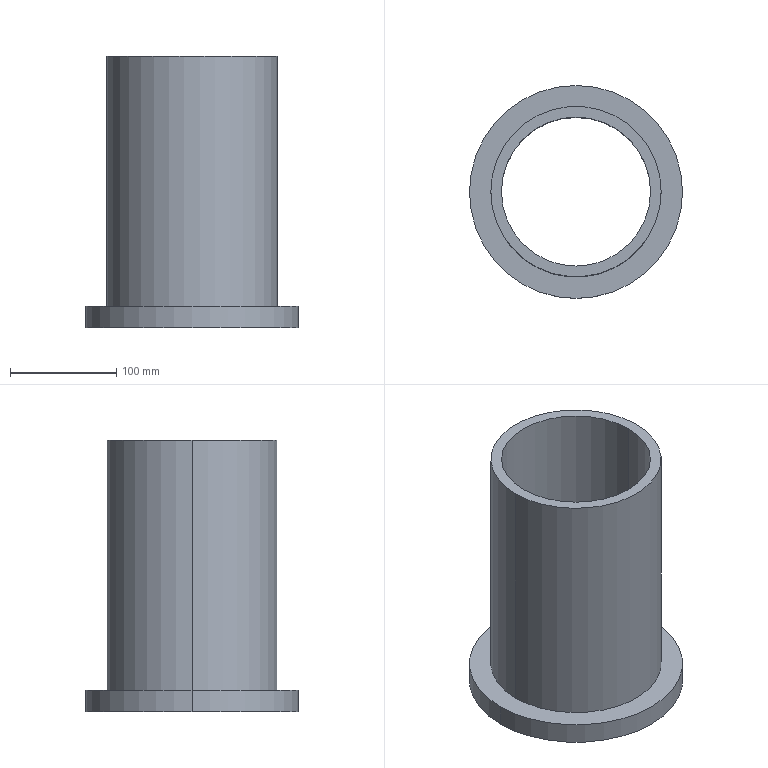Part | SolidWorks | features BaseBody 1 | 1 solid | 9 faces | box 200 x 200 x 255 mm | volume 1427854 mm3 | cylinder 6 | plane 3 | commonest cylinder face diameters 140 x2 160 x2 200 x2
STEP:
#1=CARTESIAN_POINT('',(335.077,953.249,-384.893));
#2=VERTEX_POINT('',#1);
#3=CARTESIAN_POINT('',(335.077,953.249,-639.893));
#4=VERTEX_POINT('',#3);
#5=CARTESIAN_POINT('',(335.077,953.249,-384.893));
#6=DIRECTION('',(0.,0.,-1.));
#7=VECTOR('',#6,1000.);
#8=LINE('',#5,#7);
#9=EDGE_CURVE('',#2,#4,#8,.T.);
#10=ORIENTED_EDGE('',*,*,#9,.F.);
#11=CARTESIAN_POINT('',(195.077,953.249,-384.893));
#12=VERTEX_POINT('',#11);
#13=CARTESIAN_POINT('',(265.077,953.249,-384.893));
#14=DIRECTION('',(0.,0.,1.));
#15=DIRECTION('',(1.,0.,0.));
#16=AXIS2_PLACEMENT_3D('',#13,#14,#15);
#17=CIRCLE('',#16,70.);
#18=EDGE_CURVE('',#2,#12,#17,.T.);
#19=ORIENTED_EDGE('',*,*,#18,.T.);
#20=CARTESIAN_POINT('',(195.077,953.249,-639.893));
#21=VERTEX_POINT('',#20);
#22=CARTESIAN_POINT('',(195.077,953.249,-384.893));
#23=DIRECTION('',(0.,0.,-1.));
#24=VECTOR('',#23,1000.);
#25=LINE('',#22,#24);
#26=EDGE_CURVE('',#12,#21,#25,.T.);
#27=ORIENTED_EDGE('',*,*,#26,.T.);
#28=CARTESIAN_POINT('',(265.077,953.249,-639.893));
#29=DIRECTION('',(0.,0.,1.));
#30=DIRECTION('',(1.,0.,0.));
#31=AXIS2_PLACEMENT_3D('',#28,#29,#30);
#32=CIRCLE('',#31,70.);
#33=EDGE_CURVE('',#4,#21,#32,.T.);
#34=ORIENTED_EDGE('',*,*,#33,.F.);
#35=EDGE_LOOP('',(#10,#19,#27,#34));
#36=FACE_OUTER_BOUND('',#35,.T.);
#37=CARTESIAN_POINT('',(265.077,953.249,-384.893));
#38=DIRECTION('',(0.,0.,-1.));
#39=DIRECTION('',(1.,0.,0.));
#40=AXIS2_PLACEMENT_3D('',#37,#38,#39);
#41=CYLINDRICAL_SURFACE('',#40,70.);
#42=ADVANCED_FACE('',(#36),#41,.F.);
#43=CARTESIAN_POINT('',(345.077,953.249,-384.893));
#44=VERTEX_POINT('',#43);
#45=CARTESIAN_POINT('',(345.077,953.249,-619.893));
#46=VERTEX_POINT('',#45);
#47=CARTESIAN_POINT('',(345.077,953.249,-384.893));
#48=DIRECTION('',(0.,0.,-1.));
#49=VECTOR('',#48,1000.);
#50=LINE('',#47,#49);
#51=EDGE_CURVE('',#44,#46,#50,.T.);
#52=ORIENTED_EDGE('',*,*,#51,.F.);
#53=CARTESIAN_POINT('',(185.077,953.249,-384.893));
#54=VERTEX_POINT('',#53);
#55=CARTESIAN_POINT('',(265.077,953.249,-384.893));
#56=DIRECTION('',(0.,0.,1.));
#57=DIRECTION('',(1.,0.,0.));
#58=AXIS2_PLACEMENT_3D('',#55,#56,#57);
#59=CIRCLE('',#58,80.);
#60=EDGE_CURVE('',#54,#44,#59,.T.);
#61=ORIENTED_EDGE('',*,*,#60,.F.);
#62=CARTESIAN_POINT('',(185.077,953.249,-619.893));
#63=VERTEX_POINT('',#62);
#64=CARTESIAN_POINT('',(185.077,953.249,-384.893));
#65=DIRECTION('',(0.,0.,-1.));
#66=VECTOR('',#65,1000.);
#67=LINE('',#64,#66);
#68=EDGE_CURVE('',#54,#63,#67,.T.);
#69=ORIENTED_EDGE('',*,*,#68,.T.);
#70=CARTESIAN_POINT('',(265.077,953.249,-619.893));
#71=DIRECTION('',(0.,0.,-1.));
#72=DIRECTION('',(1.,0.,0.));
#73=AXIS2_PLACEMENT_3D('',#70,#71,#72);
#74=CIRCLE('',#73,80.);
#75=EDGE_CURVE('',#46,#63,#74,.T.);
#76=ORIENTED_EDGE('',*,*,#75,.F.);
#77=EDGE_LOOP('',(#52,#61,#69,#76));
#78=FACE_OUTER_BOUND('',#77,.T.);
#79=CARTESIAN_POINT('',(265.077,953.249,-384.893));
#80=DIRECTION('',(0.,0.,-1.));
#81=DIRECTION('',(1.,0.,0.));
#82=AXIS2_PLACEMENT_3D('',#79,#80,#81);
#83=CYLINDRICAL_SURFACE('',#82,80.);
#84=ADVANCED_FACE('',(#78),#83,.T.);
#85=CARTESIAN_POINT('',(265.077,953.249,-384.893));
#86=DIRECTION('',(0.,0.,1.));
#87=DIRECTION('',(1.,0.,0.));
#88=AXIS2_PLACEMENT_3D('',#85,#86,#87);
#89=CIRCLE('',#88,70.);
#90=EDGE_CURVE('',#12,#2,#89,.T.);
#91=ORIENTED_EDGE('',*,*,#90,.F.);
#92=ORIENTED_EDGE('',*,*,#18,.F.);
#93=EDGE_LOOP('',(#91,#92));
#94=FACE_BOUND('',#93,.T.);
#95=ORIENTED_EDGE('',*,*,#60,.T.);
#96=CARTESIAN_POINT('',(265.077,953.249,-384.893));
#97=DIRECTION('',(0.,0.,1.));
#98=DIRECTION('',(1.,0.,0.));
#99=AXIS2_PLACEMENT_3D('',#96,#97,#98);
#100=CIRCLE('',#99,80.);
#101=EDGE_CURVE('',#44,#54,#100,.T.);
#102=ORIENTED_EDGE('',*,*,#101,.T.);
#103=EDGE_LOOP('',(#95,#102));
#104=FACE_OUTER_BOUND('',#103,.T.);
#105=CARTESIAN_POINT('',(265.077,953.249,-384.893));
#106=DIRECTION('',(0.,0.,1.));
#107=DIRECTION('',(1.,0.,0.));
#108=AXIS2_PLACEMENT_3D('',#105,#106,#107);
#109=PLANE('',#108);
#110=ADVANCED_FACE('',(#94,#104),#109,.T.);
#111=CARTESIAN_POINT('',(365.077,953.249,-619.893));
#112=VERTEX_POINT('',#111);
#113=CARTESIAN_POINT('',(365.077,953.249,-639.893));
#114=VERTEX_POINT('',#113);
#115=CARTESIAN_POINT('',(365.077,953.249,-619.893));
#116=DIRECTION('',(0.,0.,-1.));
#117=VECTOR('',#116,1000.);
#118=LINE('',#115,#117);
#119=EDGE_CURVE('',#112,#114,#118,.T.);
#120=ORIENTED_EDGE('',*,*,#119,.F.);
#121=CARTESIAN_POINT('',(165.077,953.249,-619.893));
#122=VERTEX_POINT('',#121);
#123=CARTESIAN_POINT('',(265.077,953.249,-619.893));
#124=DIRECTION('',(0.,0.,1.));
#125=DIRECTION('',(1.,0.,0.));
#126=AXIS2_PLACEMENT_3D('',#123,#124,#125);
#127=CIRCLE('',#126,100.);
#128=EDGE_CURVE('',#122,#112,#127,.T.);
#129=ORIENTED_EDGE('',*,*,#128,.F.);
#130=CARTESIAN_POINT('',(165.077,953.249,-639.893));
#131=VERTEX_POINT('',#130);
#132=CARTESIAN_POINT('',(165.077,953.249,-619.893));
#133=DIRECTION('',(0.,0.,-1.));
#134=VECTOR('',#133,1000.);
#135=LINE('',#132,#134);
#136=EDGE_CURVE('',#122,#131,#135,.T.);
#137=ORIENTED_EDGE('',*,*,#136,.T.);
#138=CARTESIAN_POINT('',(265.077,953.249,-639.893));
#139=DIRECTION('',(0.,0.,1.));
#140=DIRECTION('',(1.,0.,0.));
#141=AXIS2_PLACEMENT_3D('',#138,#139,#140);
#142=CIRCLE('',#141,100.);
#143=EDGE_CURVE('',#131,#114,#142,.T.);
#144=ORIENTED_EDGE('',*,*,#143,.T.);
#145=EDGE_LOOP('',(#120,#129,#137,#144));
#146=FACE_OUTER_BOUND('',#145,.T.);
#147=CARTESIAN_POINT('',(265.077,953.249,-619.893));
#148=DIRECTION('',(0.,0.,-1.));
#149=DIRECTION('',(1.,0.,0.));
#150=AXIS2_PLACEMENT_3D('',#147,#148,#149);
#151=CYLINDRICAL_SURFACE('',#150,100.);
#152=ADVANCED_FACE('',(#146),#151,.T.);
#153=CARTESIAN_POINT('',(265.077,953.249,-619.893));
#154=DIRECTION('',(0.,0.,-1.));
#155=DIRECTION('',(1.,0.,0.));
#156=AXIS2_PLACEMENT_3D('',#153,#154,#155);
#157=CIRCLE('',#156,80.);
#158=EDGE_CURVE('',#63,#46,#157,.T.);
#159=ORIENTED_EDGE('',*,*,#158,.T.);
#160=ORIENTED_EDGE('',*,*,#75,.T.);
#161=EDGE_LOOP('',(#159,#160));
#162=FACE_BOUND('',#161,.T.);
#163=ORIENTED_EDGE('',*,*,#128,.T.);
#164=CARTESIAN_POINT('',(265.077,953.249,-619.893));
#165=DIRECTION('',(0.,0.,1.));
#166=DIRECTION('',(1.,0.,0.));
#167=AXIS2_PLACEMENT_3D('',#164,#165,#166);
#168=CIRCLE('',#167,100.);
#169=EDGE_CURVE('',#112,#122,#168,.T.);
#170=ORIENTED_EDGE('',*,*,#169,.T.);
#171=EDGE_LOOP('',(#163,#170));
#172=FACE_OUTER_BOUND('',#171,.T.);
#173=CARTESIAN_POINT('',(265.077,953.249,-619.893));
#174=DIRECTION('',(0.,0.,1.));
#175=DIRECTION('',(1.,0.,0.));
#176=AXIS2_PLACEMENT_3D('',#173,#174,#175);
#177=PLANE('',#176);
#178=ADVANCED_FACE('',(#162,#172),#177,.T.);
#179=CARTESIAN_POINT('',(265.077,953.249,-639.893));
#180=DIRECTION('',(0.,0.,1.));
#181=DIRECTION('',(1.,0.,0.));
#182=AXIS2_PLACEMENT_3D('',#179,#180,#181);
#183=CIRCLE('',#182,70.);
#184=EDGE_CURVE('',#21,#4,#183,.T.);
#185=ORIENTED_EDGE('',*,*,#184,.T.);
#186=ORIENTED_EDGE('',*,*,#33,.T.);
#187=EDGE_LOOP('',(#185,#186));
#188=FACE_BOUND('',#187,.T.);
#189=ORIENTED_EDGE('',*,*,#143,.F.);
#190=CARTESIAN_POINT('',(265.077,953.249,-639.893));
#191=DIRECTION('',(0.,0.,1.));
#192=DIRECTION('',(1.,0.,0.));
#193=AXIS2_PLACEMENT_3D('',#190,#191,#192);
#194=CIRCLE('',#193,100.);
#195=EDGE_CURVE('',#114,#131,#194,.T.);
#196=ORIENTED_EDGE('',*,*,#195,.F.);
#197=EDGE_LOOP('',(#189,#196));
#198=FACE_OUTER_BOUND('',#197,.T.);
#199=CARTESIAN_POINT('',(265.077,953.249,-639.893));
#200=DIRECTION('',(0.,0.,1.));
#201=DIRECTION('',(1.,0.,0.));
#202=AXIS2_PLACEMENT_3D('',#199,#200,#201);
#203=PLANE('',#202);
#204=ADVANCED_FACE('',(#188,#198),#203,.F.);
#205=ORIENTED_EDGE('',*,*,#169,.F.);
#206=ORIENTED_EDGE('',*,*,#119,.T.);
#207=ORIENTED_EDGE('',*,*,#195,.T.);
#208=ORIENTED_EDGE('',*,*,#136,.F.);
#209=EDGE_LOOP('',(#205,#206,#207,#208));
#210=FACE_OUTER_BOUND('',#209,.T.);
#211=CARTESIAN_POINT('',(265.077,953.249,-619.893));
#212=DIRECTION('',(0.,0.,-1.));
#213=DIRECTION('',(1.,0.,0.));
#214=AXIS2_PLACEMENT_3D('',#211,#212,#213);
#215=CYLINDRICAL_SURFACE('',#214,100.);
#216=ADVANCED_FACE('',(#210),#215,.T.);
#217=ORIENTED_EDGE('',*,*,#101,.F.);
#218=ORIENTED_EDGE('',*,*,#51,.T.);
#219=ORIENTED_EDGE('',*,*,#158,.F.);
#220=ORIENTED_EDGE('',*,*,#68,.F.);
#221=EDGE_LOOP('',(#217,#218,#219,#220));
#222=FACE_OUTER_BOUND('',#221,.T.);
#223=CARTESIAN_POINT('',(265.077,953.249,-384.893));
#224=DIRECTION('',(0.,0.,-1.));
#225=DIRECTION('',(1.,0.,0.));
#226=AXIS2_PLACEMENT_3D('',#223,#224,#225);
#227=CYLINDRICAL_SURFACE('',#226,80.);
#228=ADVANCED_FACE('',(#222),#227,.T.);
#229=ORIENTED_EDGE('',*,*,#90,.T.);
#230=ORIENTED_EDGE('',*,*,#9,.T.);
#231=ORIENTED_EDGE('',*,*,#184,.F.);
#232=ORIENTED_EDGE('',*,*,#26,.F.);
#233=EDGE_LOOP('',(#229,#230,#231,#232));
#234=FACE_OUTER_BOUND('',#233,.T.);
#235=CARTESIAN_POINT('',(265.077,953.249,-384.893));
#236=DIRECTION('',(0.,0.,-1.));
#237=DIRECTION('',(1.,0.,0.));
#238=AXIS2_PLACEMENT_3D('',#235,#236,#237);
#239=CYLINDRICAL_SURFACE('',#238,70.);
#240=ADVANCED_FACE('',(#234),#239,.F.);
#241=CLOSED_SHELL('',(#42,#84,#110,#152,#178,#204,#216,#228,#240));
#242=MANIFOLD_SOLID_BREP('',#241);
#243=CARTESIAN_POINT('',(0.,0.,0.));
#244=DIRECTION('',(0.,0.,1.));
#245=DIRECTION('',(1.,0.,0.));
#246=AXIS2_PLACEMENT_3D('',#243,#244,#245);
#247=(LENGTH_UNIT()NAMED_UNIT(*)SI_UNIT(.MILLI.,.METRE.));
#248=UNCERTAINTY_MEASURE_WITH_UNIT(LENGTH_MEASURE(0.00001),#247,'','');
#249=(NAMED_UNIT(*)PLANE_ANGLE_UNIT()SI_UNIT($,.RADIAN.));
#250=(NAMED_UNIT(*)SI_UNIT($,.STERADIAN.)SOLID_ANGLE_UNIT());
#251=(GEOMETRIC_REPRESENTATION_CONTEXT(3)GLOBAL_UNCERTAINTY_ASSIGNED_CONTEXT((#248))GLOBAL_UNIT_ASSIGNED_CONTEXT((#247,#249,#250))REPRESENTATION_CONTEXT('',''));
#252=ADVANCED_BREP_SHAPE_REPRESENTATION('',(#242,#246),#251);